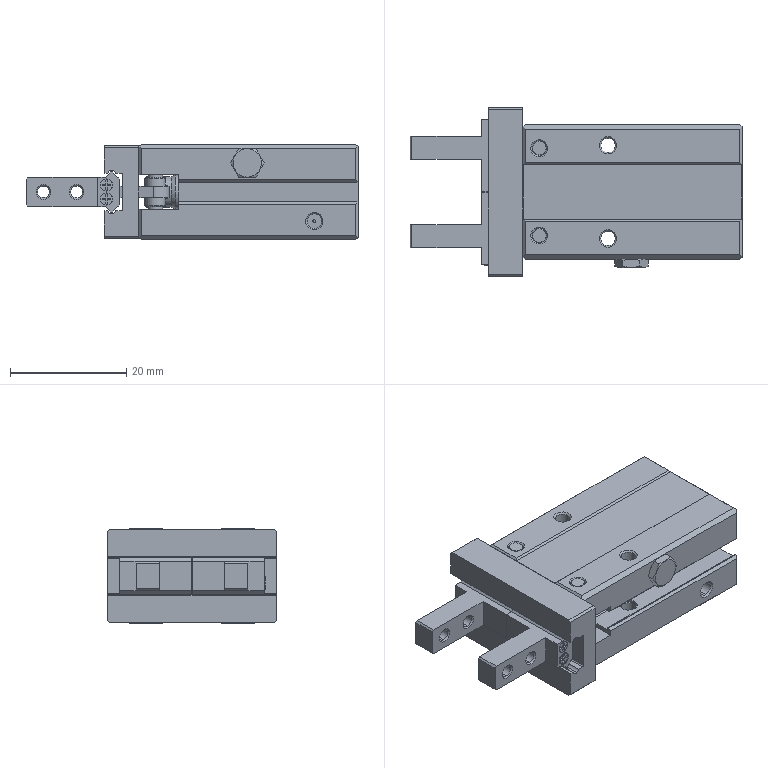Part | STEP file | HFSZ10-CL-G-11 | 1 solid | 441 faces | box 57 x 29 x 16.4 mm | volume 14404 mm3 | plane 224 | cylinder 138 | cone 71 | spline 8 | commonest cylinder face diameters 2.459 x20 0.4 x14 2 x10 0.27 x8 2.013 x8 2.1 x8